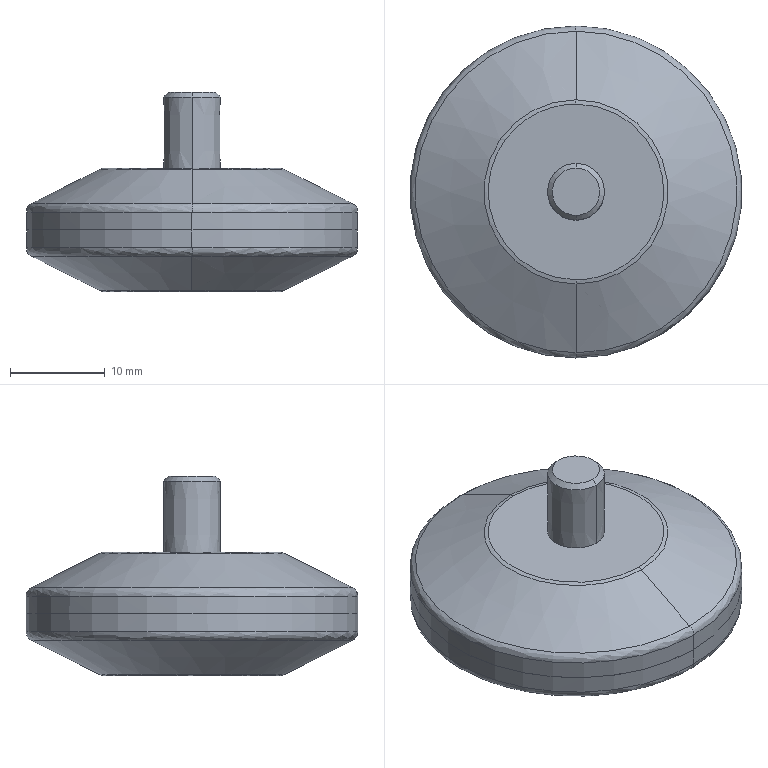Part | SolidWorks | features BaseBody 1 | 1 solid | 24 faces | box 35 x 35 x 21 mm | volume 9731 mm3 | spline 8 | cone 8 | cylinder 4 | plane 4 | commonest cylinder face diameters 34.99 x2 35 x2
STEP:
#1=CARTESIAN_POINT('',(480.537,55.215,-89.852));
#2=VERTEX_POINT('',#1);
#3=CARTESIAN_POINT('',(480.461,55.215,-89.852));
#4=VERTEX_POINT('',#3);
#5=CARTESIAN_POINT('',(480.537,37.715,-89.852));
#6=DIRECTION('',(0.000000001,-0.000000003,1.));
#7=DIRECTION('',(0.004352,-1.,-0.000000003));
#8=AXIS2_PLACEMENT_3D('',#5,#6,#7);
#9=CIRCLE('',#8,17.5);
#10=EDGE_CURVE('',#2,#4,#9,.T.);
#11=ORIENTED_EDGE('',*,*,#10,.T.);
#12=CARTESIAN_POINT('',(480.463,54.662,-88.958));
#13=VERTEX_POINT('',#12);
#14=CARTESIAN_POINT('',(480.465,54.215,-89.852));
#15=DIRECTION('',(1.,0.004352,-0.000000001));
#16=DIRECTION('',(-0.004352,1.,0.000000003));
#17=AXIS2_PLACEMENT_3D('',#14,#15,#16);
#18=CIRCLE('',#17,1.);
#19=EDGE_CURVE('',#4,#13,#18,.T.);
#20=ORIENTED_EDGE('',*,*,#19,.T.);
#21=CARTESIAN_POINT('',(480.537,54.662,-88.958));
#22=VERTEX_POINT('',#21);
#23=CARTESIAN_POINT('',(480.537,37.715,-88.958));
#24=DIRECTION('',(0.000000001,-0.000000003,1.));
#25=DIRECTION('',(0.004352,-1.,-0.000000003));
#26=AXIS2_PLACEMENT_3D('',#23,#24,#25);
#27=CIRCLE('',#26,16.947);
#28=EDGE_CURVE('',#22,#13,#27,.T.);
#29=ORIENTED_EDGE('',*,*,#28,.F.);
#30=CARTESIAN_POINT('',(480.611,20.768,-88.958));
#31=VERTEX_POINT('',#30);
#32=CARTESIAN_POINT('',(480.537,37.715,-88.958));
#33=DIRECTION('',(0.000000001,-0.000000003,1.));
#34=DIRECTION('',(0.004352,-1.,-0.000000003));
#35=AXIS2_PLACEMENT_3D('',#32,#33,#34);
#36=CIRCLE('',#35,16.947);
#37=EDGE_CURVE('',#31,#22,#36,.T.);
#38=ORIENTED_EDGE('',*,*,#37,.F.);
#39=CARTESIAN_POINT('',(480.613,20.215,-89.852));
#40=VERTEX_POINT('',#39);
#41=CARTESIAN_POINT('',(480.609,21.215,-89.852));
#42=DIRECTION('',(-1.,-0.004352,0.000000001));
#43=DIRECTION('',(0.004352,-1.,-0.000000003));
#44=AXIS2_PLACEMENT_3D('',#41,#42,#43);
#45=CIRCLE('',#44,1.);
#46=EDGE_CURVE('',#40,#31,#45,.T.);
#47=ORIENTED_EDGE('',*,*,#46,.F.);
#48=CARTESIAN_POINT('',(480.537,37.715,-89.852));
#49=DIRECTION('',(0.000000001,-0.000000003,1.));
#50=DIRECTION('',(0.004352,-1.,-0.000000003));
#51=AXIS2_PLACEMENT_3D('',#48,#49,#50);
#52=CIRCLE('',#51,17.5);
#53=EDGE_CURVE('',#40,#2,#52,.T.);
#54=ORIENTED_EDGE('',*,*,#53,.T.);
#55=EDGE_LOOP('',(#11,#20,#29,#38,#47,#54));
#56=FACE_OUTER_BOUND('',#55,.T.);
#57=CARTESIAN_POINT('',(480.461,55.215,-89.852));
#58=CARTESIAN_POINT('',(515.46,55.367,-89.852));
#59=CARTESIAN_POINT('',(515.613,20.367,-89.852));
#60=CARTESIAN_POINT('',(480.613,20.215,-89.852));
#61=CARTESIAN_POINT('',(480.461,55.215,-89.463));
#62=CARTESIAN_POINT('',(515.46,55.367,-89.463));
#63=CARTESIAN_POINT('',(515.613,20.367,-89.463));
#64=CARTESIAN_POINT('',(480.613,20.215,-89.463));
#65=CARTESIAN_POINT('',(480.462,55.01,-89.132));
#66=CARTESIAN_POINT('',(515.052,55.16,-89.132));
#67=CARTESIAN_POINT('',(515.203,20.57,-89.132));
#68=CARTESIAN_POINT('',(480.612,20.42,-89.132));
#69=CARTESIAN_POINT('',(480.463,54.662,-88.958));
#70=CARTESIAN_POINT('',(514.357,54.809,-88.958));
#71=CARTESIAN_POINT('',(514.505,20.915,-88.958));
#72=CARTESIAN_POINT('',(480.611,20.768,-88.958));
#73=(BOUNDED_SURFACE()B_SPLINE_SURFACE(3,3,((#57,#58,#59,#60),(#61,#62,#63,#64),(#65,#66,#67,#68),(#69,#70,#71,#72)),.UNSPECIFIED.,.F.,.F.,.F.)B_SPLINE_SURFACE_WITH_KNOTS((4,4),(4,4),(0.,1.),(0.,1.),.UNSPECIFIED.)GEOMETRIC_REPRESENTATION_ITEM()RATIONAL_B_SPLINE_SURFACE(((1.,0.3333,0.3333,1.),(0.9004,0.3001,0.3001,0.9004),(0.9004,0.3001,0.3001,0.9004),(1.,0.3333,0.3333,1.)))REPRESENTATION_ITEM('')SURFACE());
#74=ADVANCED_FACE('',(#56),#73,.T.);
#75=CARTESIAN_POINT('',(480.577,28.451,-85.234));
#76=VERTEX_POINT('',#75);
#77=CARTESIAN_POINT('',(480.497,46.979,-85.234));
#78=VERTEX_POINT('',#77);
#79=CARTESIAN_POINT('',(480.577,28.451,-85.234));
#80=CARTESIAN_POINT('',(462.049,28.37,-85.234));
#81=CARTESIAN_POINT('',(461.969,46.898,-85.234));
#82=CARTESIAN_POINT('',(480.497,46.979,-85.234));
#83=(BOUNDED_CURVE()B_SPLINE_CURVE(3,(#79,#80,#81,#82),.UNSPECIFIED.,.F.,.F.)B_SPLINE_CURVE_WITH_KNOTS((4,4),(0.,1.),.UNSPECIFIED.)CURVE()GEOMETRIC_REPRESENTATION_ITEM()RATIONAL_B_SPLINE_CURVE((1.,0.3333,0.3333,1.))REPRESENTATION_ITEM(''));
#84=EDGE_CURVE('',#76,#78,#83,.T.);
#85=ORIENTED_EDGE('',*,*,#84,.T.);
#86=CARTESIAN_POINT('',(480.495,47.426,-85.34));
#87=VERTEX_POINT('',#86);
#88=CARTESIAN_POINT('',(480.497,46.979,-86.234));
#89=DIRECTION('',(-1.,-0.004352,0.000000001));
#90=DIRECTION('',(-0.004352,1.,0.000000003));
#91=AXIS2_PLACEMENT_3D('',#88,#89,#90);
#92=CIRCLE('',#91,1.);
#93=EDGE_CURVE('',#78,#87,#92,.T.);
#94=ORIENTED_EDGE('',*,*,#93,.T.);
#95=CARTESIAN_POINT('',(480.537,28.004,-85.34));
#96=VERTEX_POINT('',#95);
#97=CARTESIAN_POINT('',(480.537,37.715,-85.34));
#98=DIRECTION('',(-0.000000001,0.000000003,-1.));
#99=DIRECTION('',(0.004352,-1.,-0.000000003));
#100=AXIS2_PLACEMENT_3D('',#97,#98,#99);
#101=CIRCLE('',#100,9.711);
#102=EDGE_CURVE('',#96,#87,#101,.T.);
#103=ORIENTED_EDGE('',*,*,#102,.F.);
#104=CARTESIAN_POINT('',(480.579,28.004,-85.34));
#105=VERTEX_POINT('',#104);
#106=CARTESIAN_POINT('',(480.537,37.715,-85.34));
#107=DIRECTION('',(-0.000000001,0.000000003,-1.));
#108=DIRECTION('',(0.004352,-1.,-0.000000003));
#109=AXIS2_PLACEMENT_3D('',#106,#107,#108);
#110=CIRCLE('',#109,9.711);
#111=EDGE_CURVE('',#105,#96,#110,.T.);
#112=ORIENTED_EDGE('',*,*,#111,.F.);
#113=CARTESIAN_POINT('',(480.577,28.451,-86.234));
#114=DIRECTION('',(1.,0.004352,-0.000000001));
#115=DIRECTION('',(0.004352,-1.,-0.000000003));
#116=AXIS2_PLACEMENT_3D('',#113,#114,#115);
#117=CIRCLE('',#116,1.);
#118=EDGE_CURVE('',#76,#105,#117,.T.);
#119=ORIENTED_EDGE('',*,*,#118,.F.);
#120=EDGE_LOOP('',(#85,#94,#103,#112,#119));
#121=FACE_OUTER_BOUND('',#120,.T.);
#122=CARTESIAN_POINT('',(480.497,46.979,-85.234));
#123=CARTESIAN_POINT('',(461.969,46.898,-85.234));
#124=CARTESIAN_POINT('',(462.049,28.37,-85.234));
#125=CARTESIAN_POINT('',(480.577,28.451,-85.234));
#126=CARTESIAN_POINT('',(480.496,47.135,-85.234));
#127=CARTESIAN_POINT('',(461.656,47.053,-85.234));
#128=CARTESIAN_POINT('',(461.738,28.213,-85.234));
#129=CARTESIAN_POINT('',(480.578,28.295,-85.234));
#130=CARTESIAN_POINT('',(480.495,47.286,-85.27));
#131=CARTESIAN_POINT('',(461.352,47.203,-85.27));
#132=CARTESIAN_POINT('',(461.435,28.06,-85.27));
#133=CARTESIAN_POINT('',(480.579,28.143,-85.27));
#134=CARTESIAN_POINT('',(480.495,47.426,-85.34));
#135=CARTESIAN_POINT('',(461.072,47.341,-85.34));
#136=CARTESIAN_POINT('',(461.157,27.919,-85.34));
#137=CARTESIAN_POINT('',(480.579,28.004,-85.34));
#138=(BOUNDED_SURFACE()B_SPLINE_SURFACE(3,3,((#122,#123,#124,#125),(#126,#127,#128,#129),(#130,#131,#132,#133),(#134,#135,#136,#137)),.UNSPECIFIED.,.F.,.F.,.F.)B_SPLINE_SURFACE_WITH_KNOTS((4,4),(4,4),(0.,1.),(0.,1.),.UNSPECIFIED.)GEOMETRIC_REPRESENTATION_ITEM()RATIONAL_B_SPLINE_SURFACE(((1.,0.3333,0.3333,1.),(0.9822,0.3274,0.3274,0.9822),(0.9822,0.3274,0.3274,0.9822),(1.,0.3333,0.3333,1.)))REPRESENTATION_ITEM('')SURFACE());
#139=ADVANCED_FACE('',(#121),#138,.T.);
#140=CARTESIAN_POINT('',(480.461,55.21,-93.616));
#141=VERTEX_POINT('',#140);
#142=CARTESIAN_POINT('',(480.537,20.22,-93.616));
#143=VERTEX_POINT('',#142);
#144=CARTESIAN_POINT('',(480.537,37.715,-93.616));
#145=DIRECTION('',(0.000000001,-0.000000003,1.));
#146=DIRECTION('',(0.,-1.,-0.000000003));
#147=AXIS2_PLACEMENT_3D('',#144,#145,#146);
#148=CIRCLE('',#147,17.495);
#149=EDGE_CURVE('',#141,#143,#148,.T.);
#150=ORIENTED_EDGE('',*,*,#149,.F.);
#151=CARTESIAN_POINT('',(480.463,54.657,-94.511));
#152=VERTEX_POINT('',#151);
#153=CARTESIAN_POINT('',(480.465,54.21,-93.616));
#154=DIRECTION('',(-1.,-0.004352,0.000000001));
#155=DIRECTION('',(-0.004352,1.,0.000000003));
#156=AXIS2_PLACEMENT_3D('',#153,#154,#155);
#157=CIRCLE('',#156,1.);
#158=EDGE_CURVE('',#141,#152,#157,.T.);
#159=ORIENTED_EDGE('',*,*,#158,.T.);
#160=CARTESIAN_POINT('',(480.537,20.772,-94.511));
#161=VERTEX_POINT('',#160);
#162=CARTESIAN_POINT('',(480.537,37.715,-94.511));
#163=DIRECTION('',(0.000000001,-0.000000003,1.));
#164=DIRECTION('',(0.004352,-1.,-0.000000003));
#165=AXIS2_PLACEMENT_3D('',#162,#163,#164);
#166=CIRCLE('',#165,16.942);
#167=EDGE_CURVE('',#152,#161,#166,.T.);
#168=ORIENTED_EDGE('',*,*,#167,.T.);
#169=CARTESIAN_POINT('',(480.611,20.773,-94.511));
#170=VERTEX_POINT('',#169);
#171=CARTESIAN_POINT('',(480.537,37.715,-94.511));
#172=DIRECTION('',(0.000000001,-0.000000003,1.));
#173=DIRECTION('',(0.004352,-1.,-0.000000003));
#174=AXIS2_PLACEMENT_3D('',#171,#172,#173);
#175=CIRCLE('',#174,16.942);
#176=EDGE_CURVE('',#161,#170,#175,.T.);
#177=ORIENTED_EDGE('',*,*,#176,.T.);
#178=CARTESIAN_POINT('',(480.613,20.22,-93.616));
#179=VERTEX_POINT('',#178);
#180=CARTESIAN_POINT('',(480.609,21.22,-93.616));
#181=DIRECTION('',(1.,0.004352,-0.000000001));
#182=DIRECTION('',(0.004352,-1.,-0.000000003));
#183=AXIS2_PLACEMENT_3D('',#180,#181,#182);
#184=CIRCLE('',#183,1.);
#185=EDGE_CURVE('',#179,#170,#184,.T.);
#186=ORIENTED_EDGE('',*,*,#185,.F.);
#187=CARTESIAN_POINT('',(480.537,37.715,-93.616));
#188=DIRECTION('',(0.000000001,-0.000000003,1.));
#189=DIRECTION('',(0.,-1.,-0.000000003));
#190=AXIS2_PLACEMENT_3D('',#187,#188,#189);
#191=CIRCLE('',#190,17.495);
#192=EDGE_CURVE('',#143,#179,#191,.T.);
#193=ORIENTED_EDGE('',*,*,#192,.F.);
#194=EDGE_LOOP('',(#150,#159,#168,#177,#186,#193));
#195=FACE_OUTER_BOUND('',#194,.T.);
#196=CARTESIAN_POINT('',(480.461,55.21,-93.616));
#197=CARTESIAN_POINT('',(445.471,55.057,-93.616));
#198=CARTESIAN_POINT('',(445.623,20.068,-93.616));
#199=CARTESIAN_POINT('',(480.613,20.22,-93.616));
#200=CARTESIAN_POINT('',(480.461,55.21,-94.005));
#201=CARTESIAN_POINT('',(445.471,55.057,-94.005));
#202=CARTESIAN_POINT('',(445.623,20.068,-94.005));
#203=CARTESIAN_POINT('',(480.613,20.22,-94.005));
#204=CARTESIAN_POINT('',(480.462,55.005,-94.336));
#205=CARTESIAN_POINT('',(445.881,54.854,-94.336));
#206=CARTESIAN_POINT('',(446.032,20.274,-94.336));
#207=CARTESIAN_POINT('',(480.612,20.425,-94.336));
#208=CARTESIAN_POINT('',(480.463,54.657,-94.511));
#209=CARTESIAN_POINT('',(446.579,54.509,-94.511));
#210=CARTESIAN_POINT('',(446.726,20.625,-94.511));
#211=CARTESIAN_POINT('',(480.611,20.773,-94.511));
#212=(BOUNDED_SURFACE()B_SPLINE_SURFACE(3,3,((#196,#197,#198,#199),(#200,#201,#202,#203),(#204,#205,#206,#207),(#208,#209,#210,#211)),.UNSPECIFIED.,.F.,.F.,.F.)B_SPLINE_SURFACE_WITH_KNOTS((4,4),(4,4),(0.,1.),(0.,1.),.UNSPECIFIED.)GEOMETRIC_REPRESENTATION_ITEM()RATIONAL_B_SPLINE_SURFACE(((1.,0.3333,0.3333,1.),(0.9004,0.3001,0.3001,0.9004),(0.9004,0.3001,0.3001,0.9004),(1.,0.3333,0.3333,1.)))REPRESENTATION_ITEM('')SURFACE());
#213=ADVANCED_FACE('',(#195),#212,.T.);
#214=CARTESIAN_POINT('',(480.577,28.456,-98.234));
#215=VERTEX_POINT('',#214);
#216=CARTESIAN_POINT('',(480.497,46.974,-98.234));
#217=VERTEX_POINT('',#216);
#218=CARTESIAN_POINT('',(480.577,28.456,-98.234));
#219=CARTESIAN_POINT('',(499.095,28.536,-98.234));
#220=CARTESIAN_POINT('',(499.014,47.054,-98.234));
#221=CARTESIAN_POINT('',(480.497,46.974,-98.234));
#222=(BOUNDED_CURVE()B_SPLINE_CURVE(3,(#218,#219,#220,#221),.UNSPECIFIED.,.F.,.F.)B_SPLINE_CURVE_WITH_KNOTS((4,4),(0.,1.),.UNSPECIFIED.)CURVE()GEOMETRIC_REPRESENTATION_ITEM()RATIONAL_B_SPLINE_CURVE((1.,0.3333,0.3333,1.))REPRESENTATION_ITEM(''));
#223=EDGE_CURVE('',#215,#217,#222,.T.);
#224=ORIENTED_EDGE('',*,*,#223,.T.);
#225=CARTESIAN_POINT('',(480.495,47.421,-98.129));
#226=VERTEX_POINT('',#225);
#227=CARTESIAN_POINT('',(480.497,46.974,-97.234));
#228=DIRECTION('',(1.,0.004352,-0.000000001));
#229=DIRECTION('',(-0.004352,1.,0.000000003));
#230=AXIS2_PLACEMENT_3D('',#227,#228,#229);
#231=CIRCLE('',#230,1.);
#232=EDGE_CURVE('',#217,#226,#231,.T.);
#233=ORIENTED_EDGE('',*,*,#232,.T.);
#234=CARTESIAN_POINT('',(480.537,47.421,-98.129));
#235=VERTEX_POINT('',#234);
#236=CARTESIAN_POINT('',(480.537,37.715,-98.129));
#237=DIRECTION('',(0.000000001,-0.000000003,1.));
#238=DIRECTION('',(0.004352,-1.,-0.000000003));
#239=AXIS2_PLACEMENT_3D('',#236,#237,#238);
#240=CIRCLE('',#239,9.706);
#241=EDGE_CURVE('',#235,#226,#240,.T.);
#242=ORIENTED_EDGE('',*,*,#241,.F.);
#243=CARTESIAN_POINT('',(480.579,28.009,-98.129));
#244=VERTEX_POINT('',#243);
#245=CARTESIAN_POINT('',(480.537,37.715,-98.129));
#246=DIRECTION('',(0.000000001,-0.000000003,1.));
#247=DIRECTION('',(0.004352,-1.,-0.000000003));
#248=AXIS2_PLACEMENT_3D('',#245,#246,#247);
#249=CIRCLE('',#248,9.706);
#250=EDGE_CURVE('',#244,#235,#249,.T.);
#251=ORIENTED_EDGE('',*,*,#250,.F.);
#252=CARTESIAN_POINT('',(480.577,28.456,-97.234));
#253=DIRECTION('',(-1.,-0.004352,0.000000001));
#254=DIRECTION('',(0.004352,-1.,-0.000000003));
#255=AXIS2_PLACEMENT_3D('',#252,#253,#254);
#256=CIRCLE('',#255,1.);
#257=EDGE_CURVE('',#215,#244,#256,.T.);
#258=ORIENTED_EDGE('',*,*,#257,.F.);
#259=EDGE_LOOP('',(#224,#233,#242,#251,#258));
#260=FACE_OUTER_BOUND('',#259,.T.);
#261=CARTESIAN_POINT('',(480.497,46.974,-98.234));
#262=CARTESIAN_POINT('',(499.014,47.054,-98.234));
#263=CARTESIAN_POINT('',(499.095,28.536,-98.234));
#264=CARTESIAN_POINT('',(480.577,28.456,-98.234));
#265=CARTESIAN_POINT('',(480.496,47.13,-98.234));
#266=CARTESIAN_POINT('',(499.325,47.211,-98.234));
#267=CARTESIAN_POINT('',(499.407,28.382,-98.234));
#268=CARTESIAN_POINT('',(480.578,28.3,-98.234));
#269=CARTESIAN_POINT('',(480.495,47.281,-98.198));
#270=CARTESIAN_POINT('',(499.628,47.365,-98.198));
#271=CARTESIAN_POINT('',(499.712,28.231,-98.198));
#272=CARTESIAN_POINT('',(480.578,28.148,-98.198));
#273=CARTESIAN_POINT('',(480.495,47.421,-98.129));
#274=CARTESIAN_POINT('',(499.907,47.505,-98.129));
#275=CARTESIAN_POINT('',(499.991,28.093,-98.129));
#276=CARTESIAN_POINT('',(480.579,28.009,-98.129));
#277=(BOUNDED_SURFACE()B_SPLINE_SURFACE(3,3,((#261,#262,#263,#264),(#265,#266,#267,#268),(#269,#270,#271,#272),(#273,#274,#275,#276)),.UNSPECIFIED.,.F.,.F.,.F.)B_SPLINE_SURFACE_WITH_KNOTS((4,4),(4,4),(0.,1.),(0.,1.),.UNSPECIFIED.)GEOMETRIC_REPRESENTATION_ITEM()RATIONAL_B_SPLINE_SURFACE(((1.,0.3333,0.3333,1.),(0.9822,0.3274,0.3274,0.9822),(0.9822,0.3274,0.3274,0.9822),(1.,0.3333,0.3333,1.)))REPRESENTATION_ITEM('')SURFACE());
#278=ADVANCED_FACE('',(#260),#277,.T.);
#279=CARTESIAN_POINT('',(480.537,47.426,-85.34));
#280=VERTEX_POINT('',#279);
#281=CARTESIAN_POINT('',(480.537,37.715,-85.34));
#282=DIRECTION('',(-0.000000001,0.000000003,-1.));
#283=DIRECTION('',(0.004352,-1.,-0.000000003));
#284=AXIS2_PLACEMENT_3D('',#281,#282,#283);
#285=CIRCLE('',#284,9.711);
#286=EDGE_CURVE('',#280,#105,#285,.T.);
#287=ORIENTED_EDGE('',*,*,#286,.T.);
#288=ORIENTED_EDGE('',*,*,#111,.T.);
#289=CARTESIAN_POINT('',(480.537,20.767,-88.958));
#290=VERTEX_POINT('',#289);
#291=CARTESIAN_POINT('',(480.537,20.767,-88.958));
#292=DIRECTION('',(0.,-0.8944,-0.4472));
#293=VECTOR('',#292,1000.);
#294=LINE('',#291,#293);
#295=EDGE_CURVE('',#96,#290,#294,.T.);
#296=ORIENTED_EDGE('',*,*,#295,.T.);
#297=CARTESIAN_POINT('',(480.537,37.715,-88.958));
#298=DIRECTION('',(0.000000001,-0.000000003,1.));
#299=DIRECTION('',(0.004352,-1.,-0.000000003));
#300=AXIS2_PLACEMENT_3D('',#297,#298,#299);
#301=CIRCLE('',#300,16.947);
#302=EDGE_CURVE('',#290,#31,#301,.T.);
#303=ORIENTED_EDGE('',*,*,#302,.T.);
#304=ORIENTED_EDGE('',*,*,#37,.T.);
#305=CARTESIAN_POINT('',(480.537,54.662,-88.958));
#306=DIRECTION('',(0.,0.8944,-0.4472));
#307=VECTOR('',#306,1000.);
#308=LINE('',#305,#307);
#309=EDGE_CURVE('',#280,#22,#308,.T.);
#310=ORIENTED_EDGE('',*,*,#309,.F.);
#311=EDGE_LOOP('',(#287,#288,#296,#303,#304,#310));
#312=FACE_OUTER_BOUND('',#311,.T.);
#313=CARTESIAN_POINT('',(480.537,37.715,-88.958));
#314=DIRECTION('',(-0.000000001,0.000000003,-1.));
#315=DIRECTION('',(0.,1.,0.000000003));
#316=AXIS2_PLACEMENT_3D('',#313,#314,#315);
#317=CONICAL_SURFACE('',#316,16.947,1.107);
#318=ADVANCED_FACE('',(#312),#317,.T.);
#319=CARTESIAN_POINT('',(480.537,20.215,-91.734));
#320=VERTEX_POINT('',#319);
#321=CARTESIAN_POINT('',(480.537,55.215,-91.734));
#322=VERTEX_POINT('',#321);
#323=CARTESIAN_POINT('',(480.537,37.715,-91.734));
#324=DIRECTION('',(0.000000001,-0.000000003,1.));
#325=DIRECTION('',(0.,-1.,-0.000000003));
#326=AXIS2_PLACEMENT_3D('',#323,#324,#325);
#327=CIRCLE('',#326,17.5);
#328=EDGE_CURVE('',#320,#322,#327,.T.);
#329=ORIENTED_EDGE('',*,*,#328,.T.);
#330=CARTESIAN_POINT('',(480.537,55.215,-85.234));
#331=DIRECTION('',(0.000000001,-0.000000003,1.));
#332=VECTOR('',#331,1000.);
#333=LINE('',#330,#332);
#334=EDGE_CURVE('',#322,#2,#333,.T.);
#335=ORIENTED_EDGE('',*,*,#334,.T.);
#336=ORIENTED_EDGE('',*,*,#53,.F.);
#337=CARTESIAN_POINT('',(480.537,20.215,-89.852));
#338=VERTEX_POINT('',#337);
#339=CARTESIAN_POINT('',(480.537,37.715,-89.852));
#340=DIRECTION('',(0.000000001,-0.000000003,1.));
#341=DIRECTION('',(0.004352,-1.,-0.000000003));
#342=AXIS2_PLACEMENT_3D('',#339,#340,#341);
#343=CIRCLE('',#342,17.5);
#344=EDGE_CURVE('',#338,#40,#343,.T.);
#345=ORIENTED_EDGE('',*,*,#344,.F.);
#346=CARTESIAN_POINT('',(480.537,20.215,-85.234));
#347=DIRECTION('',(0.000000001,-0.000000003,1.));
#348=VECTOR('',#347,1000.);
#349=LINE('',#346,#348);
#350=EDGE_CURVE('',#320,#338,#349,.T.);
#351=ORIENTED_EDGE('',*,*,#350,.F.);
#352=EDGE_LOOP('',(#329,#335,#336,#345,#351));
#353=FACE_OUTER_BOUND('',#352,.T.);
#354=CARTESIAN_POINT('',(480.537,37.715,-85.234));
#355=DIRECTION('',(0.000000001,-0.000000003,1.));
#356=DIRECTION('',(0.,-1.,-0.000000003));
#357=AXIS2_PLACEMENT_3D('',#354,#355,#356);
#358=CYLINDRICAL_SURFACE('',#357,17.5);
#359=ADVANCED_FACE('',(#353),#358,.T.);
#360=CARTESIAN_POINT('',(480.537,40.713,-77.734));
#361=VERTEX_POINT('',#360);
#362=CARTESIAN_POINT('',(480.537,34.716,-77.734));
#363=VERTEX_POINT('',#362);
#364=CARTESIAN_POINT('',(480.537,37.715,-77.734));
#365=DIRECTION('',(-0.000000001,0.000000003,-1.));
#366=DIRECTION('',(-0.004352,1.,0.000000003));
#367=AXIS2_PLACEMENT_3D('',#364,#365,#366);
#368=CIRCLE('',#367,2.999);
#369=EDGE_CURVE('',#361,#363,#368,.T.);
#370=ORIENTED_EDGE('',*,*,#369,.T.);
#371=CARTESIAN_POINT('',(480.537,34.715,-85.234));
#372=VERTEX_POINT('',#371);
#373=CARTESIAN_POINT('',(480.537,34.715,-85.234));
#374=DIRECTION('',(-0.000000001,-0.0001745,-1.));
#375=VECTOR('',#374,1000.);
#376=LINE('',#373,#375);
#377=EDGE_CURVE('',#363,#372,#376,.T.);
#378=ORIENTED_EDGE('',*,*,#377,.T.);
#379=CARTESIAN_POINT('',(480.537,40.715,-85.234));
#380=VERTEX_POINT('',#379);
#381=CARTESIAN_POINT('',(480.537,37.715,-85.234));
#382=DIRECTION('',(0.000000001,-0.000000003,1.));
#383=DIRECTION('',(0.,1.,0.000000003));
#384=AXIS2_PLACEMENT_3D('',#381,#382,#383);
#385=CIRCLE('',#384,3.);
#386=EDGE_CURVE('',#372,#380,#385,.T.);
#387=ORIENTED_EDGE('',*,*,#386,.T.);
#388=CARTESIAN_POINT('',(480.537,40.715,-85.234));
#389=DIRECTION('',(-0.000000001,0.0001745,-1.));
#390=VECTOR('',#389,1000.);
#391=LINE('',#388,#390);
#392=EDGE_CURVE('',#361,#380,#391,.T.);
#393=ORIENTED_EDGE('',*,*,#392,.F.);
#394=EDGE_LOOP('',(#370,#378,#387,#393));
#395=FACE_OUTER_BOUND('',#394,.T.);
#396=CARTESIAN_POINT('',(480.537,37.715,-85.234));
#397=DIRECTION('',(-0.000000001,0.000000003,-1.));
#398=DIRECTION('',(0.,1.,0.000000003));
#399=AXIS2_PLACEMENT_3D('',#396,#397,#398);
#400=CONICAL_SURFACE('',#399,3.,0.0001745);
#401=ADVANCED_FACE('',(#395),#400,.T.);
#402=ORIENTED_EDGE('',*,*,#192,.T.);
#403=CARTESIAN_POINT('',(480.537,55.21,-93.616));
#404=VERTEX_POINT('',#403);
#405=CARTESIAN_POINT('',(480.537,37.715,-93.616));
#406=DIRECTION('',(0.000000001,-0.000000003,1.));
#407=DIRECTION('',(0.,-1.,-0.000000003));
#408=AXIS2_PLACEMENT_3D('',#405,#406,#407);
#409=CIRCLE('',#408,17.495);
#410=EDGE_CURVE('',#179,#404,#409,.T.);
#411=ORIENTED_EDGE('',*,*,#410,.T.);
#412=CARTESIAN_POINT('',(480.537,55.21,-91.734));
#413=VERTEX_POINT('',#412);
#414=CARTESIAN_POINT('',(480.537,55.21,-91.734));
#415=DIRECTION('',(0.000000001,-0.000000003,1.));
#416=VECTOR('',#415,1000.);
#417=LINE('',#414,#416);
#418=EDGE_CURVE('',#404,#413,#417,.T.);
#419=ORIENTED_EDGE('',*,*,#418,.T.);
#420=CARTESIAN_POINT('',(480.537,20.22,-91.734));
#421=VERTEX_POINT('',#420);
#422=CARTESIAN_POINT('',(480.537,37.715,-91.734));
#423=DIRECTION('',(0.000000001,-0.000000003,1.));
#424=DIRECTION('',(0.,-1.,-0.000000003));
#425=AXIS2_PLACEMENT_3D('',#422,#423,#424);
#426=CIRCLE('',#425,17.495);
#427=EDGE_CURVE('',#421,#413,#426,.T.);
#428=ORIENTED_EDGE('',*,*,#427,.F.);
#429=CARTESIAN_POINT('',(480.537,20.22,-91.734));
#430=DIRECTION('',(0.000000001,-0.000000003,1.));
#431=VECTOR('',#430,1000.);
#432=LINE('',#429,#431);
#433=EDGE_CURVE('',#143,#421,#432,.T.);
#434=ORIENTED_EDGE('',*,*,#433,.F.);
#435=EDGE_LOOP('',(#402,#411,#419,#428,#434));
#436=FACE_OUTER_BOUND('',#435,.T.);
#437=CARTESIAN_POINT('',(480.537,37.715,-91.734));
#438=DIRECTION('',(0.000000001,-0.000000003,1.));
#439=DIRECTION('',(0.,-1.,-0.000000003));
#440=AXIS2_PLACEMENT_3D('',#437,#438,#439);
#441=CYLINDRICAL_SURFACE('',#440,17.495);
#442=ADVANCED_FACE('',(#436),#441,.T.);
#443=CARTESIAN_POINT('',(480.537,40.213,-77.234));
#444=VERTEX_POINT('',#443);
#445=CARTESIAN_POINT('',(480.537,35.216,-77.234));
#446=VERTEX_POINT('',#445);
#447=CARTESIAN_POINT('',(480.537,37.715,-77.234));
#448=DIRECTION('',(-0.000000001,0.000000003,-1.));
#449=DIRECTION('',(0.,1.,0.000000003));
#450=AXIS2_PLACEMENT_3D('',#447,#448,#449);
#451=CIRCLE('',#450,2.499);
#452=EDGE_CURVE('',#444,#446,#451,.T.);
#453=ORIENTED_EDGE('',*,*,#452,.T.);
#454=CARTESIAN_POINT('',(480.537,34.716,-77.734));
#455=DIRECTION('',(-0.000000001,-0.7072,-0.707));
#456=VECTOR('',#455,1000.);
#457=LINE('',#454,#456);
#458=EDGE_CURVE('',#446,#363,#457,.T.);
#459=ORIENTED_EDGE('',*,*,#458,.T.);
#460=ORIENTED_EDGE('',*,*,#369,.F.);
#461=CARTESIAN_POINT('',(480.537,40.713,-77.734));
#462=DIRECTION('',(-0.000000001,0.7072,-0.707));
#463=VECTOR('',#462,1000.);
#464=LINE('',#461,#463);
#465=EDGE_CURVE('',#444,#361,#464,.T.);
#466=ORIENTED_EDGE('',*,*,#465,.F.);
#467=EDGE_LOOP('',(#453,#459,#460,#466));
#468=FACE_OUTER_BOUND('',#467,.T.);
#469=CARTESIAN_POINT('',(480.537,37.715,-77.734));
#470=DIRECTION('',(-0.000000001,0.000000003,-1.));
#471=DIRECTION('',(0.,1.,0.000000003));
#472=AXIS2_PLACEMENT_3D('',#469,#470,#471);
#473=CONICAL_SURFACE('',#472,2.999,0.7855);
#474=ADVANCED_FACE('',(#468),#473,.T.);
#475=CARTESIAN_POINT('',(480.537,28.009,-98.129));
#476=VERTEX_POINT('',#475);
#477=CARTESIAN_POINT('',(480.537,37.715,-98.129));
#478=DIRECTION('',(0.000000001,-0.000000003,1.));
#479=DIRECTION('',(0.004352,-1.,-0.000000003));
#480=AXIS2_PLACEMENT_3D('',#477,#478,#479);
#481=CIRCLE('',#480,9.706);
#482=EDGE_CURVE('',#476,#244,#481,.T.);
#483=ORIENTED_EDGE('',*,*,#482,.T.);
#484=ORIENTED_EDGE('',*,*,#250,.T.);
#485=CARTESIAN_POINT('',(480.537,54.657,-94.511));
#486=VERTEX_POINT('',#485);
#487=CARTESIAN_POINT('',(480.537,54.657,-94.511));
#488=DIRECTION('',(0.,0.8944,0.4472));
#489=VECTOR('',#488,1000.);
#490=LINE('',#487,#489);
#491=EDGE_CURVE('',#235,#486,#490,.T.);
#492=ORIENTED_EDGE('',*,*,#491,.T.);
#493=CARTESIAN_POINT('',(480.537,37.715,-94.511));
#494=DIRECTION('',(0.000000001,-0.000000003,1.));
#495=DIRECTION('',(0.004352,-1.,-0.000000003));
#496=AXIS2_PLACEMENT_3D('',#493,#494,#495);
#497=CIRCLE('',#496,16.942);
#498=EDGE_CURVE('',#170,#486,#497,.T.);
#499=ORIENTED_EDGE('',*,*,#498,.F.);
#500=ORIENTED_EDGE('',*,*,#176,.F.);
#501=CARTESIAN_POINT('',(480.537,20.772,-94.511));
#502=DIRECTION('',(0.,-0.8944,0.4472));
#503=VECTOR('',#502,1000.);
#504=LINE('',#501,#503);
#505=EDGE_CURVE('',#476,#161,#504,.T.);
#506=ORIENTED_EDGE('',*,*,#505,.F.);
#507=EDGE_LOOP('',(#483,#484,#492,#499,#500,#506));
#508=FACE_OUTER_BOUND('',#507,.T.);
#509=CARTESIAN_POINT('',(480.537,37.715,-94.511));
#510=DIRECTION('',(0.000000001,-0.000000003,1.));
#511=DIRECTION('',(0.,-1.,-0.000000003));
#512=AXIS2_PLACEMENT_3D('',#509,#510,#511);
#513=CONICAL_SURFACE('',#512,16.942,1.107);
#514=ADVANCED_FACE('',(#508),#513,.T.);
#515=ORIENTED_EDGE('',*,*,#295,.F.);
#516=ORIENTED_EDGE('',*,*,#102,.T.);
#517=CARTESIAN_POINT('',(480.537,37.715,-85.34));
#518=DIRECTION('',(-0.000000001,0.000000003,-1.));
#519=DIRECTION('',(0.004352,-1.,-0.000000003));
#520=AXIS2_PLACEMENT_3D('',#517,#518,#519);
#521=CIRCLE('',#520,9.711);
#522=EDGE_CURVE('',#87,#280,#521,.T.);
#523=ORIENTED_EDGE('',*,*,#522,.T.);
#524=ORIENTED_EDGE('',*,*,#309,.T.);
#525=ORIENTED_EDGE('',*,*,#28,.T.);
#526=CARTESIAN_POINT('',(480.537,37.715,-88.958));
#527=DIRECTION('',(0.000000001,-0.000000003,1.));
#528=DIRECTION('',(0.004352,-1.,-0.000000003));
#529=AXIS2_PLACEMENT_3D('',#526,#527,#528);
#530=CIRCLE('',#529,16.947);
#531=EDGE_CURVE('',#13,#290,#530,.T.);
#532=ORIENTED_EDGE('',*,*,#531,.T.);
#533=EDGE_LOOP('',(#515,#516,#523,#524,#525,#532));
#534=FACE_OUTER_BOUND('',#533,.T.);
#535=CARTESIAN_POINT('',(480.537,37.715,-88.958));
#536=DIRECTION('',(-0.000000001,0.000000003,-1.));
#537=DIRECTION('',(0.,1.,0.000000003));
#538=AXIS2_PLACEMENT_3D('',#535,#536,#537);
#539=CONICAL_SURFACE('',#538,16.947,1.107);
#540=ADVANCED_FACE('',(#534),#539,.T.);
#541=ORIENTED_EDGE('',*,*,#19,.F.);
#542=CARTESIAN_POINT('',(480.537,37.715,-89.852));
#543=DIRECTION('',(0.000000001,-0.000000003,1.));
#544=DIRECTION('',(0.004352,-1.,-0.000000003));
#545=AXIS2_PLACEMENT_3D('',#542,#543,#544);
#546=CIRCLE('',#545,17.5);
#547=EDGE_CURVE('',#4,#338,#546,.T.);
#548=ORIENTED_EDGE('',*,*,#547,.T.);
#549=ORIENTED_EDGE('',*,*,#344,.T.);
#550=ORIENTED_EDGE('',*,*,#46,.T.);
#551=ORIENTED_EDGE('',*,*,#302,.F.);
#552=ORIENTED_EDGE('',*,*,#531,.F.);
#553=EDGE_LOOP('',(#541,#548,#549,#550,#551,#552));
#554=FACE_OUTER_BOUND('',#553,.T.);
#555=CARTESIAN_POINT('',(480.613,20.215,-89.852));
#556=CARTESIAN_POINT('',(445.613,20.063,-89.852));
#557=CARTESIAN_POINT('',(445.461,55.062,-89.852));
#558=CARTESIAN_POINT('',(480.461,55.215,-89.852));
#559=CARTESIAN_POINT('',(480.613,20.215,-89.463));
#560=CARTESIAN_POINT('',(445.613,20.063,-89.463));
#561=CARTESIAN_POINT('',(445.461,55.062,-89.463));
#562=CARTESIAN_POINT('',(480.461,55.215,-89.463));
#563=CARTESIAN_POINT('',(480.612,20.42,-89.132));
#564=CARTESIAN_POINT('',(446.022,20.269,-89.132));
#565=CARTESIAN_POINT('',(445.871,54.859,-89.132));
#566=CARTESIAN_POINT('',(480.462,55.01,-89.132));
#567=CARTESIAN_POINT('',(480.611,20.768,-88.958));
#568=CARTESIAN_POINT('',(446.717,20.62,-88.958));
#569=CARTESIAN_POINT('',(446.569,54.514,-88.958));
#570=CARTESIAN_POINT('',(480.463,54.662,-88.958));
#571=(BOUNDED_SURFACE()B_SPLINE_SURFACE(3,3,((#555,#556,#557,#558),(#559,#560,#561,#562),(#563,#564,#565,#566),(#567,#568,#569,#570)),.UNSPECIFIED.,.F.,.F.,.F.)B_SPLINE_SURFACE_WITH_KNOTS((4,4),(4,4),(0.,1.),(0.,1.),.UNSPECIFIED.)GEOMETRIC_REPRESENTATION_ITEM()RATIONAL_B_SPLINE_SURFACE(((1.,0.3333,0.3333,1.),(0.9004,0.3001,0.3001,0.9004),(0.9004,0.3001,0.3001,0.9004),(1.,0.3333,0.3333,1.)))REPRESENTATION_ITEM('')SURFACE());
#572=ADVANCED_FACE('',(#554),#571,.T.);
#573=ORIENTED_EDGE('',*,*,#93,.F.);
#574=CARTESIAN_POINT('',(480.497,46.979,-85.234));
#575=CARTESIAN_POINT('',(499.024,47.059,-85.234));
#576=CARTESIAN_POINT('',(499.105,28.532,-85.234));
#577=CARTESIAN_POINT('',(480.577,28.451,-85.234));
#578=(BOUNDED_CURVE()B_SPLINE_CURVE(3,(#574,#575,#576,#577),.UNSPECIFIED.,.F.,.F.)B_SPLINE_CURVE_WITH_KNOTS((4,4),(0.,1.),.UNSPECIFIED.)CURVE()GEOMETRIC_REPRESENTATION_ITEM()RATIONAL_B_SPLINE_CURVE((1.,0.3333,0.3333,1.))REPRESENTATION_ITEM(''));
#579=EDGE_CURVE('',#78,#76,#578,.T.);
#580=ORIENTED_EDGE('',*,*,#579,.T.);
#581=ORIENTED_EDGE('',*,*,#118,.T.);
#582=ORIENTED_EDGE('',*,*,#286,.F.);
#583=ORIENTED_EDGE('',*,*,#522,.F.);
#584=EDGE_LOOP('',(#573,#580,#581,#582,#583));
#585=FACE_OUTER_BOUND('',#584,.T.);
#586=CARTESIAN_POINT('',(480.577,28.451,-85.234));
#587=CARTESIAN_POINT('',(499.105,28.532,-85.234));
#588=CARTESIAN_POINT('',(499.024,47.059,-85.234));
#589=CARTESIAN_POINT('',(480.497,46.979,-85.234));
#590=CARTESIAN_POINT('',(480.578,28.295,-85.234));
#591=CARTESIAN_POINT('',(499.417,28.377,-85.234));
#592=CARTESIAN_POINT('',(499.335,47.216,-85.234));
#593=CARTESIAN_POINT('',(480.496,47.135,-85.234));
#594=CARTESIAN_POINT('',(480.579,28.143,-85.27));
#595=CARTESIAN_POINT('',(499.722,28.226,-85.27));
#596=CARTESIAN_POINT('',(499.638,47.37,-85.27));
#597=CARTESIAN_POINT('',(480.495,47.286,-85.27));
#598=CARTESIAN_POINT('',(480.579,28.004,-85.34));
#599=CARTESIAN_POINT('',(500.001,28.088,-85.34));
#600=CARTESIAN_POINT('',(499.917,47.51,-85.34));
#601=CARTESIAN_POINT('',(480.495,47.426,-85.34));
#602=(BOUNDED_SURFACE()B_SPLINE_SURFACE(3,3,((#586,#587,#588,#589),(#590,#591,#592,#593),(#594,#595,#596,#597),(#598,#599,#600,#601)),.UNSPECIFIED.,.F.,.F.,.F.)B_SPLINE_SURFACE_WITH_KNOTS((4,4),(4,4),(0.,1.),(0.,1.),.UNSPECIFIED.)GEOMETRIC_REPRESENTATION_ITEM()RATIONAL_B_SPLINE_SURFACE(((1.,0.3333,0.3333,1.),(0.9822,0.3274,0.3274,0.9822),(0.9822,0.3274,0.3274,0.9822),(1.,0.3333,0.3333,1.)))REPRESENTATION_ITEM('')SURFACE());
#603=ADVANCED_FACE('',(#585),#602,.T.);
#604=ORIENTED_EDGE('',*,*,#334,.F.);
#605=CARTESIAN_POINT('',(480.537,37.715,-91.734));
#606=DIRECTION('',(0.000000001,-0.000000003,1.));
#607=DIRECTION('',(0.,-1.,-0.000000003));
#608=AXIS2_PLACEMENT_3D('',#605,#606,#607);
#609=CIRCLE('',#608,17.5);
#610=EDGE_CURVE('',#322,#320,#609,.T.);
#611=ORIENTED_EDGE('',*,*,#610,.T.);
#612=ORIENTED_EDGE('',*,*,#350,.T.);
#613=ORIENTED_EDGE('',*,*,#547,.F.);
#614=ORIENTED_EDGE('',*,*,#10,.F.);
#615=EDGE_LOOP('',(#604,#611,#612,#613,#614));
#616=FACE_OUTER_BOUND('',#615,.T.);
#617=CARTESIAN_POINT('',(480.537,37.715,-85.234));
#618=DIRECTION('',(0.000000001,-0.000000003,1.));
#619=DIRECTION('',(0.,-1.,-0.000000003));
#620=AXIS2_PLACEMENT_3D('',#617,#618,#619);
#621=CYLINDRICAL_SURFACE('',#620,17.5);
#622=ADVANCED_FACE('',(#616),#621,.T.);
#623=ORIENTED_EDGE('',*,*,#84,.F.);
#624=ORIENTED_EDGE('',*,*,#579,.F.);
#625=EDGE_LOOP('',(#623,#624));
#626=FACE_OUTER_BOUND('',#625,.T.);
#627=CARTESIAN_POINT('',(480.537,37.715,-85.234));
#628=DIRECTION('',(0.000000001,-0.000000003,1.));
#629=DIRECTION('',(0.,1.,0.000000003));
#630=AXIS2_PLACEMENT_3D('',#627,#628,#629);
#631=CIRCLE('',#630,3.);
#632=EDGE_CURVE('',#380,#372,#631,.T.);
#633=ORIENTED_EDGE('',*,*,#632,.F.);
#634=ORIENTED_EDGE('',*,*,#386,.F.);
#635=EDGE_LOOP('',(#633,#634));
#636=FACE_BOUND('',#635,.T.);
#637=CARTESIAN_POINT('',(480.537,37.715,-85.234));
#638=DIRECTION('',(-0.000000001,0.000000003,-1.));
#639=DIRECTION('',(0.,1.,0.000000003));
#640=AXIS2_PLACEMENT_3D('',#637,#638,#639);
#641=PLANE('',#640);
#642=ADVANCED_FACE('',(#626,#636),#641,.F.);
#643=ORIENTED_EDGE('',*,*,#328,.F.);
#644=ORIENTED_EDGE('',*,*,#610,.F.);
#645=EDGE_LOOP('',(#643,#644));
#646=FACE_OUTER_BOUND('',#645,.T.);
#647=ORIENTED_EDGE('',*,*,#427,.T.);
#648=CARTESIAN_POINT('',(480.537,37.715,-91.734));
#649=DIRECTION('',(0.000000001,-0.000000003,1.));
#650=DIRECTION('',(0.,-1.,-0.000000003));
#651=AXIS2_PLACEMENT_3D('',#648,#649,#650);
#652=CIRCLE('',#651,17.495);
#653=EDGE_CURVE('',#413,#421,#652,.T.);
#654=ORIENTED_EDGE('',*,*,#653,.T.);
#655=EDGE_LOOP('',(#647,#654));
#656=FACE_BOUND('',#655,.T.);
#657=CARTESIAN_POINT('',(480.537,37.715,-91.734));
#658=DIRECTION('',(-0.000000001,0.000000003,-1.));
#659=DIRECTION('',(0.,1.,0.000000003));
#660=AXIS2_PLACEMENT_3D('',#657,#658,#659);
#661=PLANE('',#660);
#662=ADVANCED_FACE('',(#646,#656),#661,.T.);
#663=ORIENTED_EDGE('',*,*,#377,.F.);
#664=CARTESIAN_POINT('',(480.537,37.715,-77.734));
#665=DIRECTION('',(-0.000000001,0.000000003,-1.));
#666=DIRECTION('',(-0.004352,1.,0.000000003));
#667=AXIS2_PLACEMENT_3D('',#664,#665,#666);
#668=CIRCLE('',#667,2.999);
#669=EDGE_CURVE('',#363,#361,#668,.T.);
#670=ORIENTED_EDGE('',*,*,#669,.T.);
#671=ORIENTED_EDGE('',*,*,#392,.T.);
#672=ORIENTED_EDGE('',*,*,#632,.T.);
#673=EDGE_LOOP('',(#663,#670,#671,#672));
#674=FACE_OUTER_BOUND('',#673,.T.);
#675=CARTESIAN_POINT('',(480.537,37.715,-85.234));
#676=DIRECTION('',(-0.000000001,0.000000003,-1.));
#677=DIRECTION('',(0.,1.,0.000000003));
#678=AXIS2_PLACEMENT_3D('',#675,#676,#677);
#679=CONICAL_SURFACE('',#678,3.,0.0001745);
#680=ADVANCED_FACE('',(#674),#679,.T.);
#681=ORIENTED_EDGE('',*,*,#418,.F.);
#682=CARTESIAN_POINT('',(480.537,37.715,-93.616));
#683=DIRECTION('',(0.000000001,-0.000000003,1.));
#684=DIRECTION('',(0.,-1.,-0.000000003));
#685=AXIS2_PLACEMENT_3D('',#682,#683,#684);
#686=CIRCLE('',#685,17.495);
#687=EDGE_CURVE('',#404,#141,#686,.T.);
#688=ORIENTED_EDGE('',*,*,#687,.T.);
#689=ORIENTED_EDGE('',*,*,#149,.T.);
#690=ORIENTED_EDGE('',*,*,#433,.T.);
#691=ORIENTED_EDGE('',*,*,#653,.F.);
#692=EDGE_LOOP('',(#681,#688,#689,#690,#691));
#693=FACE_OUTER_BOUND('',#692,.T.);
#694=CARTESIAN_POINT('',(480.537,37.715,-91.734));
#695=DIRECTION('',(0.000000001,-0.000000003,1.));
#696=DIRECTION('',(0.,-1.,-0.000000003));
#697=AXIS2_PLACEMENT_3D('',#694,#695,#696);
#698=CYLINDRICAL_SURFACE('',#697,17.495);
#699=ADVANCED_FACE('',(#693),#698,.T.);
#700=ORIENTED_EDGE('',*,*,#458,.F.);
#701=CARTESIAN_POINT('',(480.537,37.715,-77.234));
#702=DIRECTION('',(-0.000000001,0.000000003,-1.));
#703=DIRECTION('',(0.,1.,0.000000003));
#704=AXIS2_PLACEMENT_3D('',#701,#702,#703);
#705=CIRCLE('',#704,2.499);
#706=EDGE_CURVE('',#446,#444,#705,.T.);
#707=ORIENTED_EDGE('',*,*,#706,.T.);
#708=ORIENTED_EDGE('',*,*,#465,.T.);
#709=ORIENTED_EDGE('',*,*,#669,.F.);
#710=EDGE_LOOP('',(#700,#707,#708,#709));
#711=FACE_OUTER_BOUND('',#710,.T.);
#712=CARTESIAN_POINT('',(480.537,37.715,-77.734));
#713=DIRECTION('',(-0.000000001,0.000000003,-1.));
#714=DIRECTION('',(0.,1.,0.000000003));
#715=AXIS2_PLACEMENT_3D('',#712,#713,#714);
#716=CONICAL_SURFACE('',#715,2.999,0.7855);
#717=ADVANCED_FACE('',(#711),#716,.T.);
#718=ORIENTED_EDGE('',*,*,#158,.F.);
#719=ORIENTED_EDGE('',*,*,#687,.F.);
#720=ORIENTED_EDGE('',*,*,#410,.F.);
#721=ORIENTED_EDGE('',*,*,#185,.T.);
#722=ORIENTED_EDGE('',*,*,#498,.T.);
#723=CARTESIAN_POINT('',(480.537,37.715,-94.511));
#724=DIRECTION('',(0.000000001,-0.000000003,1.));
#725=DIRECTION('',(0.004352,-1.,-0.000000003));
#726=AXIS2_PLACEMENT_3D('',#723,#724,#725);
#727=CIRCLE('',#726,16.942);
#728=EDGE_CURVE('',#486,#152,#727,.T.);
#729=ORIENTED_EDGE('',*,*,#728,.T.);
#730=EDGE_LOOP('',(#718,#719,#720,#721,#722,#729));
#731=FACE_OUTER_BOUND('',#730,.T.);
#732=CARTESIAN_POINT('',(480.613,20.22,-93.616));
#733=CARTESIAN_POINT('',(515.603,20.372,-93.616));
#734=CARTESIAN_POINT('',(515.45,55.362,-93.616));
#735=CARTESIAN_POINT('',(480.461,55.21,-93.616));
#736=CARTESIAN_POINT('',(480.613,20.22,-94.005));
#737=CARTESIAN_POINT('',(515.603,20.372,-94.005));
#738=CARTESIAN_POINT('',(515.45,55.362,-94.005));
#739=CARTESIAN_POINT('',(480.461,55.21,-94.005));
#740=CARTESIAN_POINT('',(480.612,20.425,-94.336));
#741=CARTESIAN_POINT('',(515.193,20.575,-94.336));
#742=CARTESIAN_POINT('',(515.042,55.155,-94.336));
#743=CARTESIAN_POINT('',(480.462,55.005,-94.336));
#744=CARTESIAN_POINT('',(480.611,20.773,-94.511));
#745=CARTESIAN_POINT('',(514.495,20.92,-94.511));
#746=CARTESIAN_POINT('',(514.347,54.804,-94.511));
#747=CARTESIAN_POINT('',(480.463,54.657,-94.511));
#748=(BOUNDED_SURFACE()B_SPLINE_SURFACE(3,3,((#732,#733,#734,#735),(#736,#737,#738,#739),(#740,#741,#742,#743),(#744,#745,#746,#747)),.UNSPECIFIED.,.F.,.F.,.F.)B_SPLINE_SURFACE_WITH_KNOTS((4,4),(4,4),(0.,1.),(0.,1.),.UNSPECIFIED.)GEOMETRIC_REPRESENTATION_ITEM()RATIONAL_B_SPLINE_SURFACE(((1.,0.3333,0.3333,1.),(0.9004,0.3001,0.3001,0.9004),(0.9004,0.3001,0.3001,0.9004),(1.,0.3333,0.3333,1.)))REPRESENTATION_ITEM('')SURFACE());
#749=ADVANCED_FACE('',(#731),#748,.T.);
#750=ORIENTED_EDGE('',*,*,#452,.F.);
#751=ORIENTED_EDGE('',*,*,#706,.F.);
#752=EDGE_LOOP('',(#750,#751));
#753=FACE_OUTER_BOUND('',#752,.T.);
#754=CARTESIAN_POINT('',(480.537,37.715,-77.234));
#755=DIRECTION('',(0.000000001,-0.000000003,1.));
#756=DIRECTION('',(0.,-1.,-0.000000003));
#757=AXIS2_PLACEMENT_3D('',#754,#755,#756);
#758=PLANE('',#757);
#759=ADVANCED_FACE('',(#753),#758,.T.);
#760=ORIENTED_EDGE('',*,*,#491,.F.);
#761=ORIENTED_EDGE('',*,*,#241,.T.);
#762=CARTESIAN_POINT('',(480.537,37.715,-98.129));
#763=DIRECTION('',(0.000000001,-0.000000003,1.));
#764=DIRECTION('',(0.004352,-1.,-0.000000003));
#765=AXIS2_PLACEMENT_3D('',#762,#763,#764);
#766=CIRCLE('',#765,9.706);
#767=EDGE_CURVE('',#226,#476,#766,.T.);
#768=ORIENTED_EDGE('',*,*,#767,.T.);
#769=ORIENTED_EDGE('',*,*,#505,.T.);
#770=ORIENTED_EDGE('',*,*,#167,.F.);
#771=ORIENTED_EDGE('',*,*,#728,.F.);
#772=EDGE_LOOP('',(#760,#761,#768,#769,#770,#771));
#773=FACE_OUTER_BOUND('',#772,.T.);
#774=CARTESIAN_POINT('',(480.537,37.715,-94.511));
#775=DIRECTION('',(0.000000001,-0.000000003,1.));
#776=DIRECTION('',(0.,-1.,-0.000000003));
#777=AXIS2_PLACEMENT_3D('',#774,#775,#776);
#778=CONICAL_SURFACE('',#777,16.942,1.107);
#779=ADVANCED_FACE('',(#773),#778,.T.);
#780=ORIENTED_EDGE('',*,*,#232,.F.);
#781=CARTESIAN_POINT('',(480.497,46.974,-98.234));
#782=CARTESIAN_POINT('',(461.979,46.893,-98.234));
#783=CARTESIAN_POINT('',(462.059,28.375,-98.234));
#784=CARTESIAN_POINT('',(480.577,28.456,-98.234));
#785=(BOUNDED_CURVE()B_SPLINE_CURVE(3,(#781,#782,#783,#784),.UNSPECIFIED.,.F.,.F.)B_SPLINE_CURVE_WITH_KNOTS((4,4),(0.,1.),.UNSPECIFIED.)CURVE()GEOMETRIC_REPRESENTATION_ITEM()RATIONAL_B_SPLINE_CURVE((1.,0.3333,0.3333,1.))REPRESENTATION_ITEM(''));
#786=EDGE_CURVE('',#217,#215,#785,.T.);
#787=ORIENTED_EDGE('',*,*,#786,.T.);
#788=ORIENTED_EDGE('',*,*,#257,.T.);
#789=ORIENTED_EDGE('',*,*,#482,.F.);
#790=ORIENTED_EDGE('',*,*,#767,.F.);
#791=EDGE_LOOP('',(#780,#787,#788,#789,#790));
#792=FACE_OUTER_BOUND('',#791,.T.);
#793=CARTESIAN_POINT('',(480.577,28.456,-98.234));
#794=CARTESIAN_POINT('',(462.059,28.375,-98.234));
#795=CARTESIAN_POINT('',(461.979,46.893,-98.234));
#796=CARTESIAN_POINT('',(480.497,46.974,-98.234));
#797=CARTESIAN_POINT('',(480.578,28.3,-98.234));
#798=CARTESIAN_POINT('',(461.748,28.218,-98.234));
#799=CARTESIAN_POINT('',(461.666,47.048,-98.234));
#800=CARTESIAN_POINT('',(480.496,47.13,-98.234));
#801=CARTESIAN_POINT('',(480.578,28.148,-98.198));
#802=CARTESIAN_POINT('',(461.445,28.065,-98.198));
#803=CARTESIAN_POINT('',(461.362,47.198,-98.198));
#804=CARTESIAN_POINT('',(480.495,47.281,-98.198));
#805=CARTESIAN_POINT('',(480.579,28.009,-98.129));
#806=CARTESIAN_POINT('',(461.167,27.924,-98.129));
#807=CARTESIAN_POINT('',(461.083,47.336,-98.129));
#808=CARTESIAN_POINT('',(480.495,47.421,-98.129));
#809=(BOUNDED_SURFACE()B_SPLINE_SURFACE(3,3,((#793,#794,#795,#796),(#797,#798,#799,#800),(#801,#802,#803,#804),(#805,#806,#807,#808)),.UNSPECIFIED.,.F.,.F.,.F.)B_SPLINE_SURFACE_WITH_KNOTS((4,4),(4,4),(0.,1.),(0.,1.),.UNSPECIFIED.)GEOMETRIC_REPRESENTATION_ITEM()RATIONAL_B_SPLINE_SURFACE(((1.,0.3333,0.3333,1.),(0.9822,0.3274,0.3274,0.9822),(0.9822,0.3274,0.3274,0.9822),(1.,0.3333,0.3333,1.)))REPRESENTATION_ITEM('')SURFACE());
#810=ADVANCED_FACE('',(#792),#809,.T.);
#811=ORIENTED_EDGE('',*,*,#786,.F.);
#812=ORIENTED_EDGE('',*,*,#223,.F.);
#813=EDGE_LOOP('',(#811,#812));
#814=FACE_OUTER_BOUND('',#813,.T.);
#815=CARTESIAN_POINT('',(480.537,37.715,-98.234));
#816=DIRECTION('',(-0.000000001,0.000000003,-1.));
#817=DIRECTION('',(0.,1.,0.000000003));
#818=AXIS2_PLACEMENT_3D('',#815,#816,#817);
#819=PLANE('',#818);
#820=ADVANCED_FACE('',(#814),#819,.T.);
#821=CLOSED_SHELL('',(#74,#139,#213,#278,#318,#359,#401,#442,#474,#514,#540,#572,#603,#622,#642,#662,#680,#699,#717,#749,#759,#779,#810,#820));
#822=MANIFOLD_SOLID_BREP('',#821);
#823=CARTESIAN_POINT('',(0.,0.,0.));
#824=DIRECTION('',(0.,0.,1.));
#825=DIRECTION('',(1.,0.,0.));
#826=AXIS2_PLACEMENT_3D('',#823,#824,#825);
#827=(LENGTH_UNIT()NAMED_UNIT(*)SI_UNIT(.MILLI.,.METRE.));
#828=UNCERTAINTY_MEASURE_WITH_UNIT(LENGTH_MEASURE(0.00001),#827,'','');
#829=(NAMED_UNIT(*)PLANE_ANGLE_UNIT()SI_UNIT($,.RADIAN.));
#830=(NAMED_UNIT(*)SI_UNIT($,.STERADIAN.)SOLID_ANGLE_UNIT());
#831=(GEOMETRIC_REPRESENTATION_CONTEXT(3)GLOBAL_UNCERTAINTY_ASSIGNED_CONTEXT((#828))GLOBAL_UNIT_ASSIGNED_CONTEXT((#827,#829,#830))REPRESENTATION_CONTEXT('',''));
#832=ADVANCED_BREP_SHAPE_REPRESENTATION('',(#822,#826),#831);